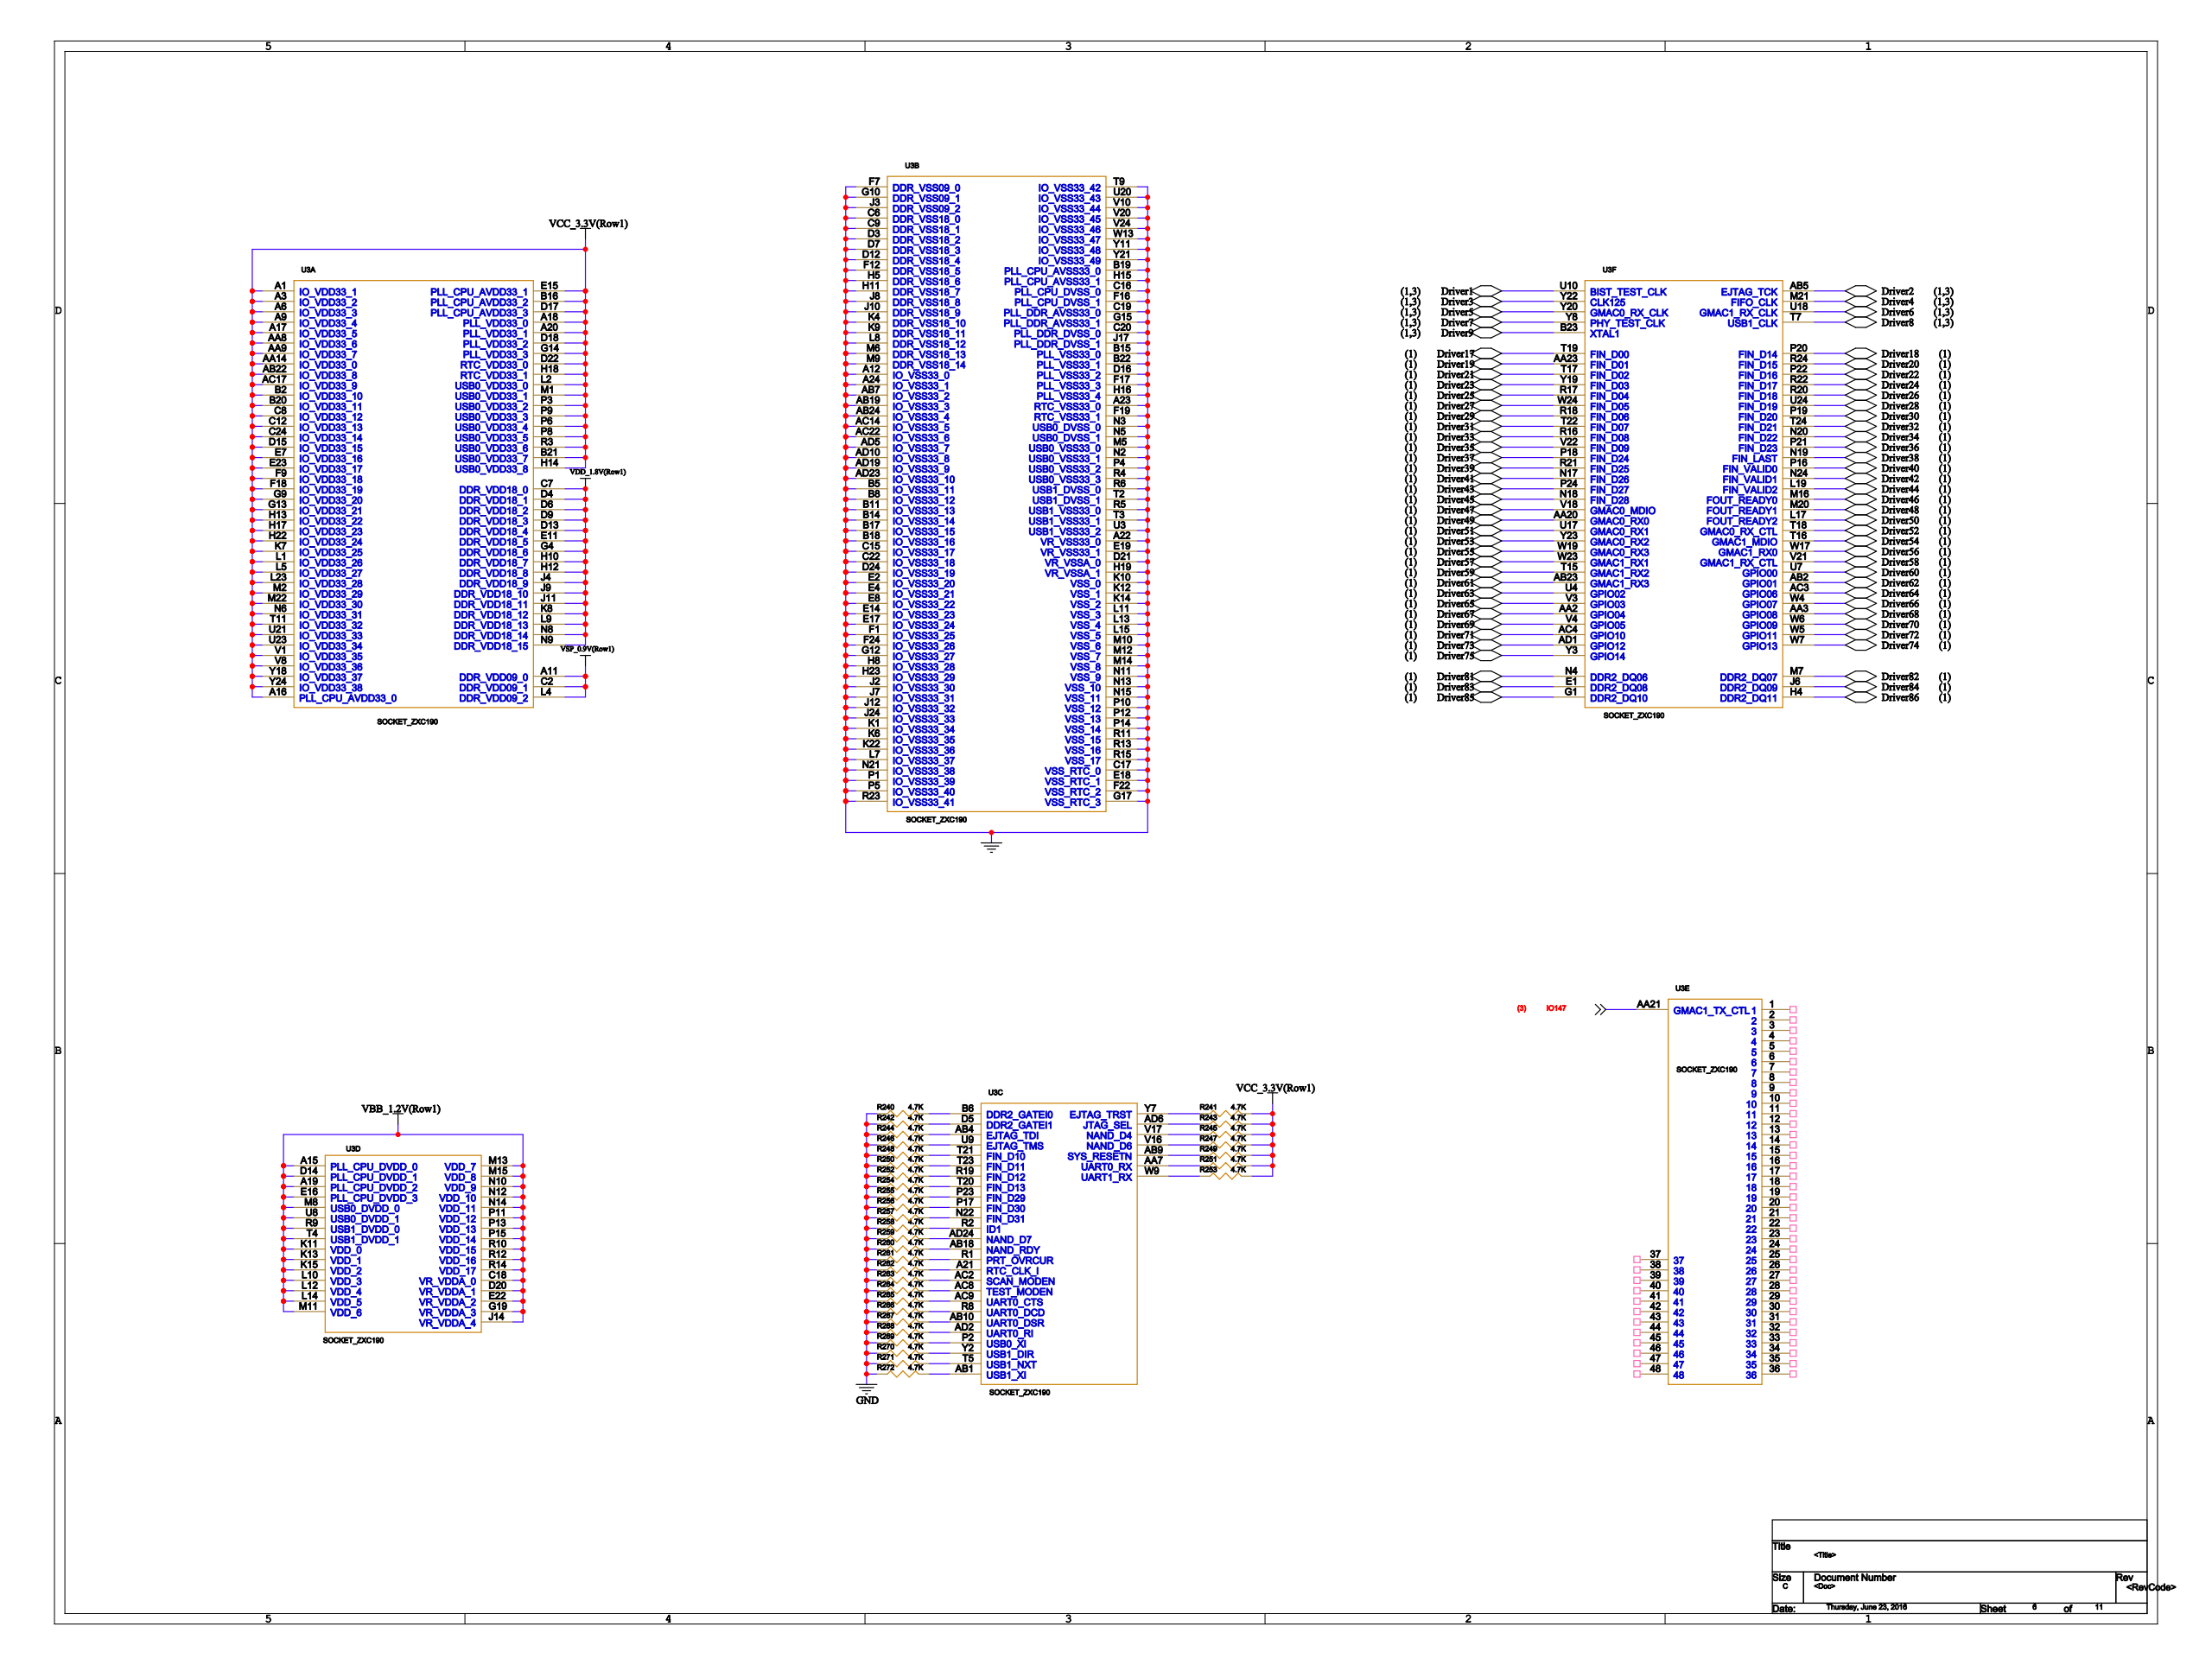Circuit board | Cadence Allegro | 531 parts | 624 nets | one sheet of the schematic
Parts on this sheet (reference | value | footprint):
R240 | 4.7K | R0805
R241 | 4.7K | R0805
R242 | 4.7K | R0805
R243 | 4.7K | R0805
R244 | 4.7K | R0805
R245 | 4.7K | R0805
R246 | 4.7K | R0805
R247 | 4.7K | R0805
R248 | 4.7K | R0805
R249 | 4.7K | R0805
R250 | 4.7K | R0805
R251 | 4.7K | R0805
R252 | 4.7K | R0805
R253 | 4.7K | R0805
R254 | 4.7K | R0805
R255 | 4.7K | R0805
R256 | 4.7K | R0805
R257 | 4.7K | R0805
R258 | 4.7K | R0805
R259 | 4.7K | R0805
R260 | 4.7K | R0805
R261 | 4.7K | R0805
R262 | 4.7K | R0805
R263 | 4.7K | R0805
R264 | 4.7K | R0805
R265 | 4.7K | R0805
R266 | 4.7K | R0805
R267 | 4.7K | R0805
R268 | 4.7K | R0805
R269 | 4.7K | R0805
R270 | 4.7K | R0805
R271 | 4.7K | R0805
R272 | 4.7K | R0805
U3 | SOCKET_ZXC190 | BGA-576
U4 | SOCKET_ZXC190 | BGA-576
U10 | SOCKET_ZXC190 | BGA-576
Nets of these parts (net: part-pin ...):
GND: R240-1 R242-1 R244-1 R246-1 R248-1 R250-1 R252-1 R254-1 R255-1 R256-1 R257-1 R258-1 R259-1 R260-1 R261-1 R262-1 R263-1 R264-1 R265-1 R266-1 R267-1 R268-1 R269-1 R270-1 R271-1 R272-1 U3-A12 U3-A22 U3-A23 U3-A24 U3-AB7 U3-AB19 U3-AB24 U3-AC14 U3-AC22 U3-AD5 U3-AD10 U3-AD19 U3-AD23 U3-B5 U3-B8 U3-B11 U3-B14 U3-B15 U3-B17 U3-B18 U3-B19 U3-B22 U3-C6 U3-C9 U3-C15 U3-C16 U3-C17 U3-C19 U3-C20 U3-C22 U3-D3 U3-D7 U3-D12 U3-D16 U3-D21 U3-D24 U3-E2 U3-E4 U3-E8 U3-E14 U3-E17 U3-E18 U3-E19 U3-F1 U3-F7 U3-F12 U3-F16 U3-F17 U3-F19 U3-F22 U3-F24 U3-G10 U3-G12 U3-G15 U3-G17 U3-H5 U3-H8 U3-H11 U3-H15 U3-H16 U3-H19 U3-H23 U3-J2 U3-J3 U3-J7 U3-J8 U3-J10 U3-J12 U3-J17 U3-J24 U3-K1 U3-K4 U3-K6 U3-K9 U3-K10 U3-K12 U3-K14 U3-K22 U3-L7 U3-L8 U3-L11 U3-L13 U3-L15 U3-M5 U3-M6 U3-M9 U3-M10 U3-M12 U3-M14 U3-N2 U3-N3 U3-N5 U3-N11 U3-N13 U3-N15 U3-N21 U3-P1 U3-P4 U3-P5 U3-P10 U3-P12 U3-P14 U3-R4 U3-R5 U3-R6 U3-R11 U3-R13 U3-R15 U3-R23 U3-T2 U3-T3 U3-T9 U3-U3 U3-U20 U3-V10 U3-V20 U3-V24 U3-W13 U3-Y11 U3-Y21 U4-A12 U4-A22 U4-A23 U4-A24 U4-AB7 U4-AB19 U4-AB24 U4-AC14 U4-AC22 U4-AD5 U4-AD10 U4-AD19 U4-AD23 U4-B5 U4-B8 U4-B11 U4-B14 U4-B15 U4-B17 U4-B18 U4-B19 U4-B22 U4-C6 U4-C9 U4-C15 U4-C16 U4-C17 U4-C19 U4-C20 U4-C22 U4-D3 U4-D7 U4-D12 U4-D16 U4-D21 U4-D24 U4-E2 U4-E4 U4-E8 U4-E14 U4-E17 U4-E18 U4-E19 U4-F1 U4-F7 U4-F12 U4-F16 U4-F17 U4-F19 U4-F22 U4-F24 U4-G10 U4-G12 U4-G15 U4-G17 U4-H5 U4-H8 U4-H11 U4-H15 U4-H16 U4-H19 U4-H23 U4-J2 U4-J3 U4-J7 U4-J8 U4-J10 U4-J12 U4-J17 U4-J24 U4-K1 U4-K4 U4-K6 U4-K9 U4-K10 U4-K12 U4-K14 U4-K22 U4-L7 U4-L8 U4-L11 U4-L13 U4-L15 U4-M5 U4-M6 U4-M9 U4-M10 U4-M12 U4-M14 U4-N2 U4-N3 U4-N5 U4-N11 U4-N13 U4-N15 U4-N21 U4-P1 U4-P4 U4-P5 U4-P10 U4-P12 U4-P14 U4-R4 U4-R5 U4-R6 U4-R11 U4-R13 U4-R15 U4-R23 U4-T2 U4-T3 U4-T9 U4-U3 U4-U20 U4-V10 U4-V20 U4-V24 U4-W13 U4-Y11 U4-Y21 U10-A12 U10-A22 U10-A23 U10-A24 U10-AB7 U10-AB19 U10-AB24 U10-AC14 U10-AC22 U10-AD5 U10-AD10 U10-AD19 U10-AD23 U10-B5 U10-B8 U10-B11 U10-B14 U10-B15 U10-B17 U10-B18 U10-B19 U10-B22 U10-C6 U10-C9 U10-C15 U10-C16 U10-C17 U10-C19 U10-C20 U10-C22 U10-D3 U10-D7 U10-D12 U10-D16 U10-D21 U10-D24 U10-E2 U10-E4 U10-E8 U10-E14 U10-E17 U10-E18 U10-E19 U10-F1 U10-F7 U10-F12 U10-F16 U10-F17 U10-F19 U10-F22 U10-F24 U10-G10 U10-G12 U10-G15 U10-G17 U10-H5 U10-H8 U10-H11 U10-H15 U10-H16 U10-H19 U10-H23 U10-J2 U10-J3 U10-J7 U10-J8 U10-J10 U10-J12 U10-J17 U10-J24 U10-K1 U10-K4 U10-K6 U10-K9 U10-K10 U10-K12 U10-K14 U10-K22 U10-L7 U10-L8 U10-L11 U10-L13 U10-L15 U10-M5 U10-M6 U10-M9 U10-M10 U10-M12 U10-M14 U10-N2 U10-N3 U10-N5 U10-N11 U10-N13 U10-N15 U10-N21 U10-P1 U10-P4 U10-P5 U10-P10 U10-P12 U10-P14 U10-R4 U10-R5 U10-R6 U10-R11 U10-R13 U10-R15 U10-R23 U10-T2 U10-T3 U10-T9 U10-U3 U10-U20 U10-V10 U10-V20 U10-V24 U10-W13 U10-Y11 U10-Y21
VCC_3.3V(ROW1): R241-2 R243-2 R245-2 R247-2 R249-2 R251-2 R253-2 U3-A1 U3-A3 U3-A6 U3-A9 U3-A16 U3-A17 U3-A18 U3-A20 U3-AA8 U3-AA9 U3-AA14 U3-AB22 U3-AC17 U3-B2 U3-B16 U3-B20 U3-B21 U3-C8 U3-C12 U3-C24 U3-D15 U3-D17 U3-D18 U3-D22 U3-E7 U3-E15 U3-E23 U3-F9 U3-F18 U3-G9 U3-G13 U3-G14 U3-H13 U3-H14 U3-H17 U3-H18 U3-H22 U3-K7 U3-L1 U3-L2 U3-L5 U3-L23 U3-M1 U3-M2 U3-M22 U3-N6 U3-P3 U3-P6 U3-P8 U3-P9 U3-R3 U3-T11 U3-U21 U3-U23 U3-V1 U3-V8 U3-Y18 U3-Y24 U4-A1 U4-A3 U4-A6 U4-A9 U4-A16 U4-A17 U4-A18 U4-A20 U4-AA8 U4-AA9 U4-AA14 U4-AB22 U4-AC17 U4-B2 U4-B16 U4-B20 U4-B21 U4-C8 U4-C12 U4-C24 U4-D15 U4-D17 U4-D18 U4-D22 U4-E7 U4-E15 U4-E23 U4-F9 U4-F18 U4-G9 U4-G13 U4-G14 U4-H13 U4-H14 U4-H17 U4-H18 U4-H22 U4-K7 U4-L1 U4-L2 U4-L5 U4-L23 U4-M1 U4-M2 U4-M22 U4-N6 U4-P3 U4-P6 U4-P8 U4-P9 U4-R3 U4-T11 U4-U21 U4-U23 U4-V1 U4-V8 U4-Y18 U4-Y24
N8545671: R240-2 U3-B6
N8546095: R241-1 U3-Y7
N8545667: R242-2 U3-D5
N8546131: R243-1 U3-AD6
N8545663: R244-2 U3-AB4
N8546275: R245-1 U3-V17
N8545659: R246-2 U3-U9
N8546279: R247-1 U3-V16
N8545655: R248-2 U3-T21
N8546303: R249-1 U3-AB9
N8545651: R250-2 U3-T23
N8546283: R251-1 U3-AA7
N8545647: R252-2 U3-R19
N8545627: R253-1 U3-W9
N8545703: R254-2 U3-T20
N8545699: R255-2 U3-P23
N8545695: R256-2 U3-P17
N8545691: R257-2 U3-N22
N8545687: R258-2 U3-R2
N8545683: R259-2 U3-AD24
N8545679: R260-2 U3-AB18
N8545675: R261-2 U3-R1
N8545731: R262-2 U3-A21
N8545727: R263-2 U3-AC2
N8545723: R264-2 U3-AC8
N8545719: R265-2 U3-AC9
N8546167: R266-2 U3-R8
N8545715: R267-2 U3-AB10
N8545711: R268-2 U3-AD2
N8545707: R269-2 U3-P2
N8545743: R270-2 U3-Y2
N8545739: R271-2 U3-T5
N8545735: R272-2 U3-AB1
IO147: U3-AA21